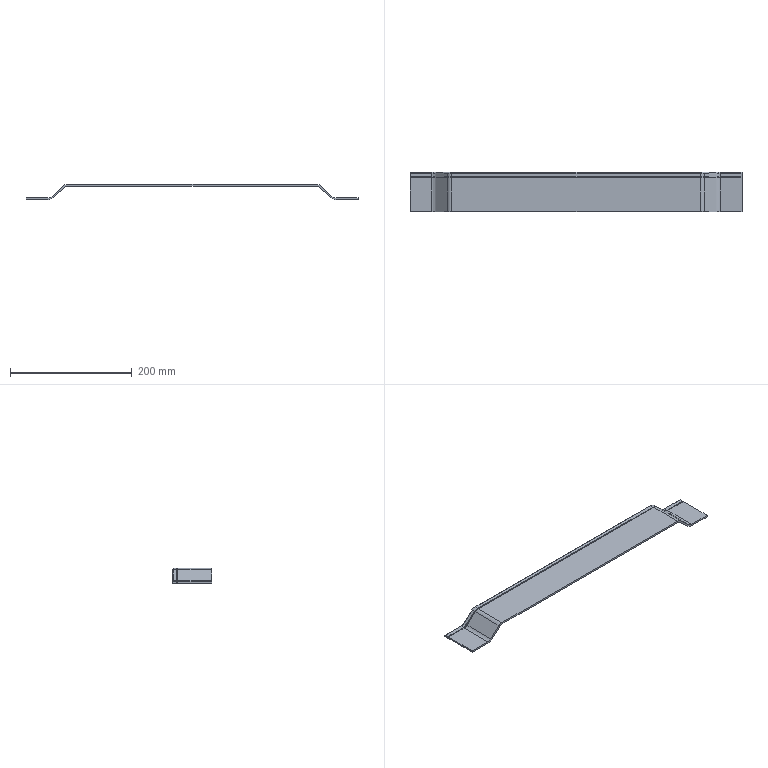Part | NX | features solid 2 | 1 solid | 93 faces | box 544.5 x 64 x 25.34 mm | volume 105928 mm3 | plane 47 | cylinder 42 | cone 4 | commonest cylinder face diameters 4 x14 6.5 x12 20 x12 14 x2 26 x2